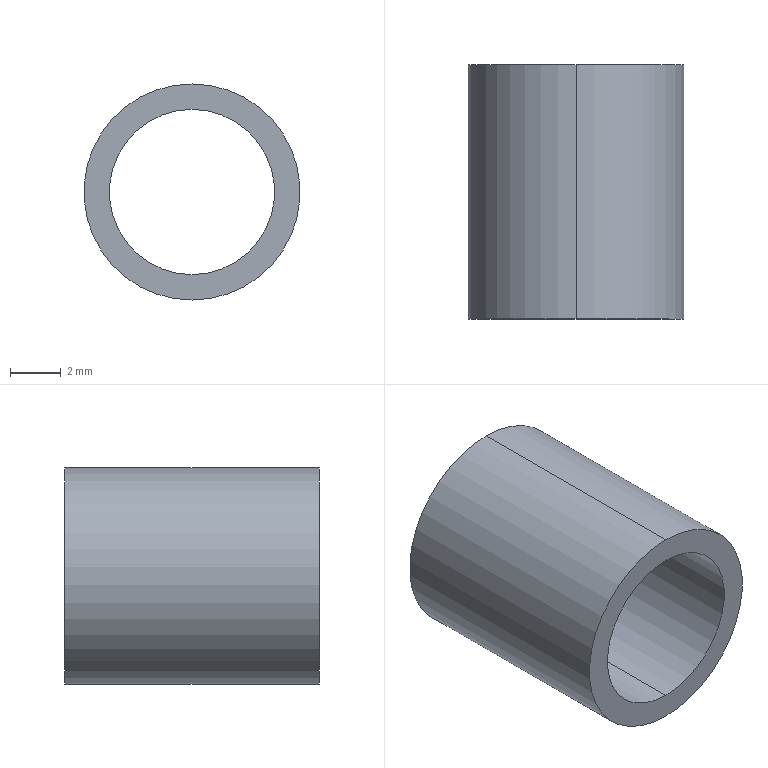Part | STEP file | joint | 1 solid | 6 faces | box 8.5 x 10 x 8.5 mm | volume 235.619 mm3 | cylinder 4 | plane 2 | commonest cylinder face diameters 6.5 x2 8.5 x2
STEP:
#1=CARTESIAN_POINT('',(0.,0.,0.));
#2=DIRECTION('',(0.,0.,1.));
#3=DIRECTION('',(1.,0.,0.));
#4=AXIS2_PLACEMENT_3D('',#1,#2,#3);
#5=CARTESIAN_POINT('',(0.,10.,-3.25));
#6=VERTEX_POINT('',#5);
#7=CARTESIAN_POINT('',(0.,0.,-3.25));
#8=VERTEX_POINT('',#7);
#9=CARTESIAN_POINT('',(0.,10.,-3.25));
#10=DIRECTION('',(0.,-1.,0.));
#11=VECTOR('',#10,1.);
#12=LINE('',#9,#11);
#13=CARTESIAN_POINT('',(0.,10.,0.));
#14=DIRECTION('',(0.,-1.,0.));
#15=DIRECTION('',(0.,0.,-1.));
#16=AXIS2_PLACEMENT_3D('',#13,#14,#15);
#17=CYLINDRICAL_SURFACE('',#16,3.25);
#18=CARTESIAN_POINT('',(6.283,0.));
#19=DIRECTION('',(0.,1.));
#20=VECTOR('',#19,1.);
#21=LINE('',#18,#20);
#22=(GEOMETRIC_REPRESENTATION_CONTEXT(2)PARAMETRIC_REPRESENTATION_CONTEXT()REPRESENTATION_CONTEXT('',''));
#23=DEFINITIONAL_REPRESENTATION('',(#21),#22);
#24=PCURVE('',#17,#23);
#25=CARTESIAN_POINT('',(0.,10.,0.));
#26=DIRECTION('',(0.,-1.,0.));
#27=DIRECTION('',(0.,0.,-1.));
#28=AXIS2_PLACEMENT_3D('',#25,#26,#27);
#29=CYLINDRICAL_SURFACE('',#28,3.25);
#30=CARTESIAN_POINT('',(0.,0.));
#31=DIRECTION('',(0.,1.));
#32=VECTOR('',#31,1.);
#33=LINE('',#30,#32);
#34=(GEOMETRIC_REPRESENTATION_CONTEXT(2)PARAMETRIC_REPRESENTATION_CONTEXT()REPRESENTATION_CONTEXT('',''));
#35=DEFINITIONAL_REPRESENTATION('',(#33),#34);
#36=PCURVE('',#29,#35);
#37=SURFACE_CURVE('',#12,(#24,#36),.PCURVE_S1.);
#38=EDGE_CURVE('',#6,#8,#37,.T.);
#39=ORIENTED_EDGE('',*,*,#38,.T.);
#40=CARTESIAN_POINT('',(0.,0.,3.25));
#41=VERTEX_POINT('',#40);
#42=CARTESIAN_POINT('',(0.,0.,0.));
#43=DIRECTION('',(0.,1.,0.));
#44=DIRECTION('',(0.,0.,1.));
#45=AXIS2_PLACEMENT_3D('',#42,#43,#44);
#46=CIRCLE('',#45,3.25);
#47=CARTESIAN_POINT('',(9.425,10.));
#48=DIRECTION('',(-1.,0.));
#49=VECTOR('',#48,1.);
#50=LINE('',#47,#49);
#51=(GEOMETRIC_REPRESENTATION_CONTEXT(2)PARAMETRIC_REPRESENTATION_CONTEXT()REPRESENTATION_CONTEXT('',''));
#52=DEFINITIONAL_REPRESENTATION('',(#50),#51);
#53=PCURVE('',#17,#52);
#54=CARTESIAN_POINT('',(0.,0.,0.));
#55=DIRECTION('',(0.,1.,0.));
#56=DIRECTION('',(0.,0.,1.));
#57=AXIS2_PLACEMENT_3D('',#54,#55,#56);
#58=PLANE('',#57);
#59=CARTESIAN_POINT('',(0.,0.));
#60=DIRECTION('',(1.,0.));
#61=AXIS2_PLACEMENT_2D('',#59,#60);
#62=CIRCLE('',#61,3.25);
#63=(GEOMETRIC_REPRESENTATION_CONTEXT(2)PARAMETRIC_REPRESENTATION_CONTEXT()REPRESENTATION_CONTEXT('',''));
#64=DEFINITIONAL_REPRESENTATION('',(#62),#63);
#65=PCURVE('',#58,#64);
#66=SURFACE_CURVE('',#46,(#53,#65),.PCURVE_S1.);
#67=EDGE_CURVE('',#8,#41,#66,.T.);
#68=ORIENTED_EDGE('',*,*,#67,.T.);
#69=CARTESIAN_POINT('',(0.,10.,3.25));
#70=VERTEX_POINT('',#69);
#71=CARTESIAN_POINT('',(0.,10.,3.25));
#72=DIRECTION('',(0.,-1.,0.));
#73=VECTOR('',#72,1.);
#74=LINE('',#71,#73);
#75=CARTESIAN_POINT('',(3.142,0.));
#76=DIRECTION('',(0.,1.));
#77=VECTOR('',#76,1.);
#78=LINE('',#75,#77);
#79=(GEOMETRIC_REPRESENTATION_CONTEXT(2)PARAMETRIC_REPRESENTATION_CONTEXT()REPRESENTATION_CONTEXT('',''));
#80=DEFINITIONAL_REPRESENTATION('',(#78),#79);
#81=PCURVE('',#17,#80);
#82=CARTESIAN_POINT('',(3.142,0.));
#83=DIRECTION('',(0.,1.));
#84=VECTOR('',#83,1.);
#85=LINE('',#82,#84);
#86=(GEOMETRIC_REPRESENTATION_CONTEXT(2)PARAMETRIC_REPRESENTATION_CONTEXT()REPRESENTATION_CONTEXT('',''));
#87=DEFINITIONAL_REPRESENTATION('',(#85),#86);
#88=PCURVE('',#29,#87);
#89=SURFACE_CURVE('',#74,(#81,#88),.PCURVE_S1.);
#90=EDGE_CURVE('',#70,#41,#89,.T.);
#91=ORIENTED_EDGE('',*,*,#90,.F.);
#92=CARTESIAN_POINT('',(0.,10.,0.));
#93=DIRECTION('',(0.,1.,0.));
#94=DIRECTION('',(0.,0.,1.));
#95=AXIS2_PLACEMENT_3D('',#92,#93,#94);
#96=CIRCLE('',#95,3.25);
#97=CARTESIAN_POINT('',(9.425,0.));
#98=DIRECTION('',(-1.,0.));
#99=VECTOR('',#98,1.);
#100=LINE('',#97,#99);
#101=(GEOMETRIC_REPRESENTATION_CONTEXT(2)PARAMETRIC_REPRESENTATION_CONTEXT()REPRESENTATION_CONTEXT('',''));
#102=DEFINITIONAL_REPRESENTATION('',(#100),#101);
#103=PCURVE('',#17,#102);
#104=CARTESIAN_POINT('',(0.,10.,0.));
#105=DIRECTION('',(0.,1.,0.));
#106=DIRECTION('',(0.,0.,1.));
#107=AXIS2_PLACEMENT_3D('',#104,#105,#106);
#108=PLANE('',#107);
#109=CARTESIAN_POINT('',(0.,0.));
#110=DIRECTION('',(1.,0.));
#111=AXIS2_PLACEMENT_2D('',#109,#110);
#112=CIRCLE('',#111,3.25);
#113=(GEOMETRIC_REPRESENTATION_CONTEXT(2)PARAMETRIC_REPRESENTATION_CONTEXT()REPRESENTATION_CONTEXT('',''));
#114=DEFINITIONAL_REPRESENTATION('',(#112),#113);
#115=PCURVE('',#108,#114);
#116=SURFACE_CURVE('',#96,(#103,#115),.PCURVE_S1.);
#117=EDGE_CURVE('',#6,#70,#116,.T.);
#118=ORIENTED_EDGE('',*,*,#117,.F.);
#119=EDGE_LOOP('',(#39,#68,#91,#118));
#120=FACE_BOUND('',#119,.F.);
#121=ADVANCED_FACE('',(#120),#17,.F.);
#122=CARTESIAN_POINT('',(0.,10.,4.25));
#123=VERTEX_POINT('',#122);
#124=CARTESIAN_POINT('',(0.,10.,-4.25));
#125=VERTEX_POINT('',#124);
#126=CARTESIAN_POINT('',(0.,10.,0.));
#127=DIRECTION('',(0.,1.,0.));
#128=DIRECTION('',(0.,0.,1.));
#129=AXIS2_PLACEMENT_3D('',#126,#127,#128);
#130=CIRCLE('',#129,4.25);
#131=CARTESIAN_POINT('',(0.,10.,0.));
#132=DIRECTION('',(0.,-1.,0.));
#133=DIRECTION('',(0.,0.,-1.));
#134=AXIS2_PLACEMENT_3D('',#131,#132,#133);
#135=CYLINDRICAL_SURFACE('',#134,4.25);
#136=CARTESIAN_POINT('',(3.142,0.));
#137=DIRECTION('',(-1.,0.));
#138=VECTOR('',#137,1.);
#139=LINE('',#136,#138);
#140=(GEOMETRIC_REPRESENTATION_CONTEXT(2)PARAMETRIC_REPRESENTATION_CONTEXT()REPRESENTATION_CONTEXT('',''));
#141=DEFINITIONAL_REPRESENTATION('',(#139),#140);
#142=PCURVE('',#135,#141);
#143=CARTESIAN_POINT('',(0.,0.));
#144=DIRECTION('',(1.,0.));
#145=AXIS2_PLACEMENT_2D('',#143,#144);
#146=CIRCLE('',#145,4.25);
#147=(GEOMETRIC_REPRESENTATION_CONTEXT(2)PARAMETRIC_REPRESENTATION_CONTEXT()REPRESENTATION_CONTEXT('',''));
#148=DEFINITIONAL_REPRESENTATION('',(#146),#147);
#149=PCURVE('',#108,#148);
#150=SURFACE_CURVE('',#130,(#142,#149),.PCURVE_S1.);
#151=EDGE_CURVE('',#123,#125,#150,.T.);
#152=ORIENTED_EDGE('',*,*,#151,.F.);
#153=CARTESIAN_POINT('',(0.,0.,4.25));
#154=VERTEX_POINT('',#153);
#155=CARTESIAN_POINT('',(0.,10.,4.25));
#156=DIRECTION('',(0.,-1.,0.));
#157=VECTOR('',#156,1.);
#158=LINE('',#155,#157);
#159=CARTESIAN_POINT('',(3.142,0.));
#160=DIRECTION('',(0.,1.));
#161=VECTOR('',#160,1.);
#162=LINE('',#159,#161);
#163=(GEOMETRIC_REPRESENTATION_CONTEXT(2)PARAMETRIC_REPRESENTATION_CONTEXT()REPRESENTATION_CONTEXT('',''));
#164=DEFINITIONAL_REPRESENTATION('',(#162),#163);
#165=PCURVE('',#135,#164);
#166=CARTESIAN_POINT('',(0.,10.,0.));
#167=DIRECTION('',(0.,-1.,0.));
#168=DIRECTION('',(0.,0.,-1.));
#169=AXIS2_PLACEMENT_3D('',#166,#167,#168);
#170=CYLINDRICAL_SURFACE('',#169,4.25);
#171=CARTESIAN_POINT('',(3.142,0.));
#172=DIRECTION('',(0.,1.));
#173=VECTOR('',#172,1.);
#174=LINE('',#171,#173);
#175=(GEOMETRIC_REPRESENTATION_CONTEXT(2)PARAMETRIC_REPRESENTATION_CONTEXT()REPRESENTATION_CONTEXT('',''));
#176=DEFINITIONAL_REPRESENTATION('',(#174),#175);
#177=PCURVE('',#170,#176);
#178=SURFACE_CURVE('',#158,(#165,#177),.PCURVE_S1.);
#179=EDGE_CURVE('',#123,#154,#178,.T.);
#180=ORIENTED_EDGE('',*,*,#179,.T.);
#181=CARTESIAN_POINT('',(0.,0.,-4.25));
#182=VERTEX_POINT('',#181);
#183=CARTESIAN_POINT('',(0.,0.,0.));
#184=DIRECTION('',(0.,1.,0.));
#185=DIRECTION('',(0.,0.,1.));
#186=AXIS2_PLACEMENT_3D('',#183,#184,#185);
#187=CIRCLE('',#186,4.25);
#188=CARTESIAN_POINT('',(3.142,10.));
#189=DIRECTION('',(-1.,0.));
#190=VECTOR('',#189,1.);
#191=LINE('',#188,#190);
#192=(GEOMETRIC_REPRESENTATION_CONTEXT(2)PARAMETRIC_REPRESENTATION_CONTEXT()REPRESENTATION_CONTEXT('',''));
#193=DEFINITIONAL_REPRESENTATION('',(#191),#192);
#194=PCURVE('',#135,#193);
#195=CARTESIAN_POINT('',(0.,0.));
#196=DIRECTION('',(1.,0.));
#197=AXIS2_PLACEMENT_2D('',#195,#196);
#198=CIRCLE('',#197,4.25);
#199=(GEOMETRIC_REPRESENTATION_CONTEXT(2)PARAMETRIC_REPRESENTATION_CONTEXT()REPRESENTATION_CONTEXT('',''));
#200=DEFINITIONAL_REPRESENTATION('',(#198),#199);
#201=PCURVE('',#58,#200);
#202=SURFACE_CURVE('',#187,(#194,#201),.PCURVE_S1.);
#203=EDGE_CURVE('',#154,#182,#202,.T.);
#204=ORIENTED_EDGE('',*,*,#203,.T.);
#205=CARTESIAN_POINT('',(0.,10.,-4.25));
#206=DIRECTION('',(0.,-1.,0.));
#207=VECTOR('',#206,1.);
#208=LINE('',#205,#207);
#209=CARTESIAN_POINT('',(0.,0.));
#210=DIRECTION('',(0.,1.));
#211=VECTOR('',#210,1.);
#212=LINE('',#209,#211);
#213=(GEOMETRIC_REPRESENTATION_CONTEXT(2)PARAMETRIC_REPRESENTATION_CONTEXT()REPRESENTATION_CONTEXT('',''));
#214=DEFINITIONAL_REPRESENTATION('',(#212),#213);
#215=PCURVE('',#135,#214);
#216=CARTESIAN_POINT('',(6.283,0.));
#217=DIRECTION('',(0.,1.));
#218=VECTOR('',#217,1.);
#219=LINE('',#216,#218);
#220=(GEOMETRIC_REPRESENTATION_CONTEXT(2)PARAMETRIC_REPRESENTATION_CONTEXT()REPRESENTATION_CONTEXT('',''));
#221=DEFINITIONAL_REPRESENTATION('',(#219),#220);
#222=PCURVE('',#170,#221);
#223=SURFACE_CURVE('',#208,(#215,#222),.PCURVE_S1.);
#224=EDGE_CURVE('',#125,#182,#223,.T.);
#225=ORIENTED_EDGE('',*,*,#224,.F.);
#226=EDGE_LOOP('',(#152,#180,#204,#225));
#227=FACE_BOUND('',#226,.T.);
#228=ADVANCED_FACE('',(#227),#135,.T.);
#229=CARTESIAN_POINT('',(0.,10.,0.));
#230=DIRECTION('',(0.,1.,0.));
#231=DIRECTION('',(0.,0.,1.));
#232=AXIS2_PLACEMENT_3D('',#229,#230,#231);
#233=CIRCLE('',#232,4.25);
#234=CARTESIAN_POINT('',(0.,0.));
#235=DIRECTION('',(1.,0.));
#236=AXIS2_PLACEMENT_2D('',#234,#235);
#237=CIRCLE('',#236,4.25);
#238=(GEOMETRIC_REPRESENTATION_CONTEXT(2)PARAMETRIC_REPRESENTATION_CONTEXT()REPRESENTATION_CONTEXT('',''));
#239=DEFINITIONAL_REPRESENTATION('',(#237),#238);
#240=PCURVE('',#108,#239);
#241=CARTESIAN_POINT('',(9.425,0.));
#242=DIRECTION('',(-1.,0.));
#243=VECTOR('',#242,1.);
#244=LINE('',#241,#243);
#245=(GEOMETRIC_REPRESENTATION_CONTEXT(2)PARAMETRIC_REPRESENTATION_CONTEXT()REPRESENTATION_CONTEXT('',''));
#246=DEFINITIONAL_REPRESENTATION('',(#244),#245);
#247=PCURVE('',#170,#246);
#248=SURFACE_CURVE('',#233,(#240,#247),.PCURVE_S1.);
#249=EDGE_CURVE('',#125,#123,#248,.T.);
#250=ORIENTED_EDGE('',*,*,#249,.T.);
#251=ORIENTED_EDGE('',*,*,#151,.T.);
#252=EDGE_LOOP('',(#250,#251));
#253=FACE_BOUND('',#252,.T.);
#254=ORIENTED_EDGE('',*,*,#117,.F.);
#255=CARTESIAN_POINT('',(0.,10.,0.));
#256=DIRECTION('',(0.,1.,0.));
#257=DIRECTION('',(0.,0.,1.));
#258=AXIS2_PLACEMENT_3D('',#255,#256,#257);
#259=CIRCLE('',#258,3.25);
#260=CARTESIAN_POINT('',(0.,0.));
#261=DIRECTION('',(1.,0.));
#262=AXIS2_PLACEMENT_2D('',#260,#261);
#263=CIRCLE('',#262,3.25);
#264=(GEOMETRIC_REPRESENTATION_CONTEXT(2)PARAMETRIC_REPRESENTATION_CONTEXT()REPRESENTATION_CONTEXT('',''));
#265=DEFINITIONAL_REPRESENTATION('',(#263),#264);
#266=PCURVE('',#108,#265);
#267=CARTESIAN_POINT('',(3.142,0.));
#268=DIRECTION('',(-1.,0.));
#269=VECTOR('',#268,1.);
#270=LINE('',#267,#269);
#271=(GEOMETRIC_REPRESENTATION_CONTEXT(2)PARAMETRIC_REPRESENTATION_CONTEXT()REPRESENTATION_CONTEXT('',''));
#272=DEFINITIONAL_REPRESENTATION('',(#270),#271);
#273=PCURVE('',#29,#272);
#274=SURFACE_CURVE('',#259,(#266,#273),.PCURVE_S1.);
#275=EDGE_CURVE('',#70,#6,#274,.T.);
#276=ORIENTED_EDGE('',*,*,#275,.F.);
#277=EDGE_LOOP('',(#254,#276));
#278=FACE_BOUND('',#277,.T.);
#279=ADVANCED_FACE('',(#253,#278),#108,.T.);
#280=CARTESIAN_POINT('',(0.,0.,0.));
#281=DIRECTION('',(0.,1.,0.));
#282=DIRECTION('',(0.,0.,1.));
#283=AXIS2_PLACEMENT_3D('',#280,#281,#282);
#284=CIRCLE('',#283,4.25);
#285=CARTESIAN_POINT('',(0.,0.));
#286=DIRECTION('',(1.,0.));
#287=AXIS2_PLACEMENT_2D('',#285,#286);
#288=CIRCLE('',#287,4.25);
#289=(GEOMETRIC_REPRESENTATION_CONTEXT(2)PARAMETRIC_REPRESENTATION_CONTEXT()REPRESENTATION_CONTEXT('',''));
#290=DEFINITIONAL_REPRESENTATION('',(#288),#289);
#291=PCURVE('',#58,#290);
#292=CARTESIAN_POINT('',(9.425,10.));
#293=DIRECTION('',(-1.,0.));
#294=VECTOR('',#293,1.);
#295=LINE('',#292,#294);
#296=(GEOMETRIC_REPRESENTATION_CONTEXT(2)PARAMETRIC_REPRESENTATION_CONTEXT()REPRESENTATION_CONTEXT('',''));
#297=DEFINITIONAL_REPRESENTATION('',(#295),#296);
#298=PCURVE('',#170,#297);
#299=SURFACE_CURVE('',#284,(#291,#298),.PCURVE_S1.);
#300=EDGE_CURVE('',#182,#154,#299,.T.);
#301=ORIENTED_EDGE('',*,*,#300,.F.);
#302=ORIENTED_EDGE('',*,*,#203,.F.);
#303=EDGE_LOOP('',(#301,#302));
#304=FACE_BOUND('',#303,.T.);
#305=ORIENTED_EDGE('',*,*,#67,.T.);
#306=CARTESIAN_POINT('',(0.,0.,0.));
#307=DIRECTION('',(0.,1.,0.));
#308=DIRECTION('',(0.,0.,1.));
#309=AXIS2_PLACEMENT_3D('',#306,#307,#308);
#310=CIRCLE('',#309,3.25);
#311=CARTESIAN_POINT('',(0.,0.));
#312=DIRECTION('',(1.,0.));
#313=AXIS2_PLACEMENT_2D('',#311,#312);
#314=CIRCLE('',#313,3.25);
#315=(GEOMETRIC_REPRESENTATION_CONTEXT(2)PARAMETRIC_REPRESENTATION_CONTEXT()REPRESENTATION_CONTEXT('',''));
#316=DEFINITIONAL_REPRESENTATION('',(#314),#315);
#317=PCURVE('',#58,#316);
#318=CARTESIAN_POINT('',(3.142,10.));
#319=DIRECTION('',(-1.,0.));
#320=VECTOR('',#319,1.);
#321=LINE('',#318,#320);
#322=(GEOMETRIC_REPRESENTATION_CONTEXT(2)PARAMETRIC_REPRESENTATION_CONTEXT()REPRESENTATION_CONTEXT('',''));
#323=DEFINITIONAL_REPRESENTATION('',(#321),#322);
#324=PCURVE('',#29,#323);
#325=SURFACE_CURVE('',#310,(#317,#324),.PCURVE_S1.);
#326=EDGE_CURVE('',#41,#8,#325,.T.);
#327=ORIENTED_EDGE('',*,*,#326,.T.);
#328=EDGE_LOOP('',(#305,#327));
#329=FACE_BOUND('',#328,.T.);
#330=ADVANCED_FACE('',(#304,#329),#58,.F.);
#331=ORIENTED_EDGE('',*,*,#179,.F.);
#332=ORIENTED_EDGE('',*,*,#249,.F.);
#333=ORIENTED_EDGE('',*,*,#224,.T.);
#334=ORIENTED_EDGE('',*,*,#300,.T.);
#335=EDGE_LOOP('',(#331,#332,#333,#334));
#336=FACE_BOUND('',#335,.T.);
#337=ADVANCED_FACE('',(#336),#170,.T.);
#338=ORIENTED_EDGE('',*,*,#326,.T.);
#339=ORIENTED_EDGE('',*,*,#38,.F.);
#340=ORIENTED_EDGE('',*,*,#275,.F.);
#341=ORIENTED_EDGE('',*,*,#90,.T.);
#342=EDGE_LOOP('',(#338,#339,#340,#341));
#343=FACE_BOUND('',#342,.F.);
#344=ADVANCED_FACE('',(#343),#29,.F.);
#345=CLOSED_SHELL('',(#121,#228,#279,#330,#337,#344));
#346=MANIFOLD_SOLID_BREP('',#345);
#347=(LENGTH_UNIT()NAMED_UNIT(*)SI_UNIT(.MILLI.,.METRE.));
#348=UNCERTAINTY_MEASURE_WITH_UNIT(LENGTH_MEASURE(0.0000001),#347,'','');
#349=(NAMED_UNIT(*)PLANE_ANGLE_UNIT()SI_UNIT($,.RADIAN.));
#350=(NAMED_UNIT(*)SI_UNIT($,.STERADIAN.)SOLID_ANGLE_UNIT());
#351=(GEOMETRIC_REPRESENTATION_CONTEXT(3)GLOBAL_UNCERTAINTY_ASSIGNED_CONTEXT((#348))GLOBAL_UNIT_ASSIGNED_CONTEXT((#347,#349,#350))REPRESENTATION_CONTEXT('',''));
#352=ADVANCED_BREP_SHAPE_REPRESENTATION('',(#4,#346),#351);